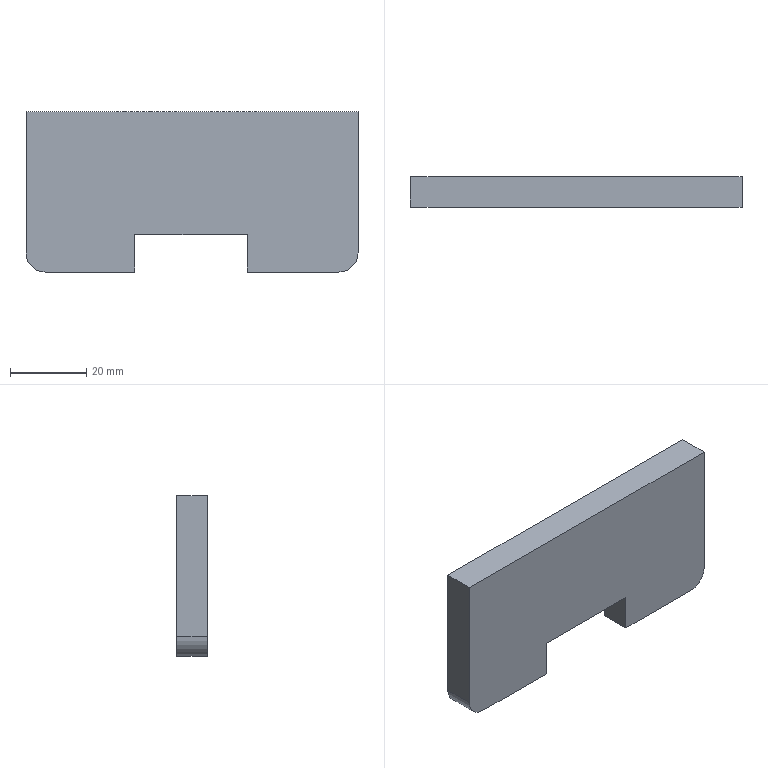Part | STEP file | 1 solid | 12 faces | box 87 x 8 x 41.949 mm | volume 26801 mm3 | plane 10 | cylinder 2 | commonest cylinder face diameters 10 x2
STEP:
#1=CARTESIAN_POINT('',(0.,0.,0.));
#2=DIRECTION('',(0.,0.,1.));
#3=DIRECTION('',(1.,0.,0.));
#4=AXIS2_PLACEMENT_3D('',#1,#2,#3);
#5=CARTESIAN_POINT('',(-4.362,37.,-78.42));
#6=VERTEX_POINT('',#5);
#7=CARTESIAN_POINT('',(-28.362,37.,-78.42));
#8=VERTEX_POINT('',#7);
#9=CARTESIAN_POINT('',(-42.862,37.,-78.42));
#10=DIRECTION('',(-1.,0.,0.));
#11=VECTOR('',#10,1.);
#12=LINE('',#9,#11);
#13=CARTESIAN_POINT('',(-42.862,37.,-64.47));
#14=DIRECTION('',(0.,1.,0.));
#15=DIRECTION('',(0.,0.,1.));
#16=AXIS2_PLACEMENT_3D('',#13,#14,#15);
#17=PLANE('',#16);
#18=CARTESIAN_POINT('',(-13.949,0.));
#19=DIRECTION('',(0.,-1.));
#20=VECTOR('',#19,1.);
#21=LINE('',#18,#20);
#22=(GEOMETRIC_REPRESENTATION_CONTEXT(2)PARAMETRIC_REPRESENTATION_CONTEXT()REPRESENTATION_CONTEXT('',''));
#23=DEFINITIONAL_REPRESENTATION('',(#21),#22);
#24=PCURVE('',#17,#23);
#25=CARTESIAN_POINT('',(-7.863,-150.,-78.42));
#26=DIRECTION('',(0.,0.,-1.));
#27=DIRECTION('',(-1.,0.,0.));
#28=AXIS2_PLACEMENT_3D('',#25,#26,#27);
#29=PLANE('',#28);
#30=CARTESIAN_POINT('',(35.,187.));
#31=DIRECTION('',(1.,0.));
#32=VECTOR('',#31,1.);
#33=LINE('',#30,#32);
#34=(GEOMETRIC_REPRESENTATION_CONTEXT(2)PARAMETRIC_REPRESENTATION_CONTEXT()REPRESENTATION_CONTEXT('',''));
#35=DEFINITIONAL_REPRESENTATION('',(#33),#34);
#36=PCURVE('',#29,#35);
#37=SURFACE_CURVE('',#12,(#24,#36),.PCURVE_S1.);
#38=EDGE_CURVE('',#6,#8,#37,.T.);
#39=ORIENTED_EDGE('',*,*,#38,.F.);
#40=CARTESIAN_POINT('',(0.6375,37.,-73.42));
#41=VERTEX_POINT('',#40);
#42=CARTESIAN_POINT('',(-4.362,37.,-73.42));
#43=DIRECTION('',(0.,-1.,0.));
#44=DIRECTION('',(0.,0.,1.));
#45=AXIS2_PLACEMENT_3D('',#42,#43,#44);
#46=CIRCLE('',#45,5.);
#47=CARTESIAN_POINT('',(-3.949,38.5));
#48=CARTESIAN_POINT('',(-3.949,29.84));
#49=CARTESIAN_POINT('',(-11.449,34.17));
#50=CARTESIAN_POINT('',(-18.949,38.5));
#51=CARTESIAN_POINT('',(-11.449,42.83));
#52=CARTESIAN_POINT('',(-3.949,47.16));
#53=CARTESIAN_POINT('',(-3.949,38.5));
#54=(BOUNDED_CURVE()B_SPLINE_CURVE(2,(#47,#48,#49,#50,#51,#52,#53),.UNSPECIFIED.,.T.,.F.)B_SPLINE_CURVE_WITH_KNOTS((1,2,2,2,2,1),(-2.094,0.,2.094,4.189,6.283,8.378),.UNSPECIFIED.)CURVE()GEOMETRIC_REPRESENTATION_ITEM()RATIONAL_B_SPLINE_CURVE((1.,0.5,1.,0.5,1.,0.5,1.))REPRESENTATION_ITEM(''));
#55=(GEOMETRIC_REPRESENTATION_CONTEXT(2)PARAMETRIC_REPRESENTATION_CONTEXT()REPRESENTATION_CONTEXT('',''));
#56=DEFINITIONAL_REPRESENTATION('',(#54),#55);
#57=PCURVE('',#17,#56);
#58=CARTESIAN_POINT('',(-4.362,37.,-73.42));
#59=DIRECTION('',(0.,-1.,0.));
#60=DIRECTION('',(0.,0.,-1.));
#61=AXIS2_PLACEMENT_3D('',#58,#59,#60);
#62=CYLINDRICAL_SURFACE('',#61,5.);
#63=CARTESIAN_POINT('',(-3.142,0.));
#64=DIRECTION('',(1.,0.));
#65=VECTOR('',#64,1.);
#66=LINE('',#63,#65);
#67=(GEOMETRIC_REPRESENTATION_CONTEXT(2)PARAMETRIC_REPRESENTATION_CONTEXT()REPRESENTATION_CONTEXT('',''));
#68=DEFINITIONAL_REPRESENTATION('',(#66),#67);
#69=PCURVE('',#62,#68);
#70=SURFACE_CURVE('',#46,(#57,#69),.PCURVE_S1.);
#71=EDGE_CURVE('',#6,#41,#70,.T.);
#72=ORIENTED_EDGE('',*,*,#71,.T.);
#73=CARTESIAN_POINT('',(0.6375,37.,-36.47));
#74=VERTEX_POINT('',#73);
#75=CARTESIAN_POINT('',(0.6375,37.,-64.47));
#76=DIRECTION('',(0.,0.,1.));
#77=VECTOR('',#76,1.);
#78=LINE('',#75,#77);
#79=CARTESIAN_POINT('',(0.,43.5));
#80=DIRECTION('',(1.,0.));
#81=VECTOR('',#80,1.);
#82=LINE('',#79,#81);
#83=(GEOMETRIC_REPRESENTATION_CONTEXT(2)PARAMETRIC_REPRESENTATION_CONTEXT()REPRESENTATION_CONTEXT('',''));
#84=DEFINITIONAL_REPRESENTATION('',(#82),#83);
#85=PCURVE('',#17,#84);
#86=CARTESIAN_POINT('',(0.6375,37.,-92.47));
#87=DIRECTION('',(-1.,0.,0.));
#88=DIRECTION('',(0.,0.,1.));
#89=AXIS2_PLACEMENT_3D('',#86,#87,#88);
#90=PLANE('',#89);
#91=CARTESIAN_POINT('',(28.,0.));
#92=DIRECTION('',(1.,0.));
#93=VECTOR('',#92,1.);
#94=LINE('',#91,#93);
#95=(GEOMETRIC_REPRESENTATION_CONTEXT(2)PARAMETRIC_REPRESENTATION_CONTEXT()REPRESENTATION_CONTEXT('',''));
#96=DEFINITIONAL_REPRESENTATION('',(#94),#95);
#97=PCURVE('',#90,#96);
#98=SURFACE_CURVE('',#78,(#85,#97),.PCURVE_S1.);
#99=EDGE_CURVE('',#41,#74,#98,.T.);
#100=ORIENTED_EDGE('',*,*,#99,.T.);
#101=CARTESIAN_POINT('',(-86.362,37.,-36.47));
#102=VERTEX_POINT('',#101);
#103=CARTESIAN_POINT('',(-42.862,37.,-36.47));
#104=DIRECTION('',(-1.,0.,0.));
#105=VECTOR('',#104,1.);
#106=LINE('',#103,#105);
#107=CARTESIAN_POINT('',(28.,0.));
#108=DIRECTION('',(0.,-1.));
#109=VECTOR('',#108,1.);
#110=LINE('',#107,#109);
#111=(GEOMETRIC_REPRESENTATION_CONTEXT(2)PARAMETRIC_REPRESENTATION_CONTEXT()REPRESENTATION_CONTEXT('',''));
#112=DEFINITIONAL_REPRESENTATION('',(#110),#111);
#113=PCURVE('',#17,#112);
#114=CARTESIAN_POINT('',(-42.862,0.,-36.47));
#115=DIRECTION('',(0.,0.,1.));
#116=DIRECTION('',(1.,0.,0.));
#117=AXIS2_PLACEMENT_3D('',#114,#115,#116);
#118=PLANE('',#117);
#119=CARTESIAN_POINT('',(0.,37.));
#120=DIRECTION('',(-1.,0.));
#121=VECTOR('',#120,1.);
#122=LINE('',#119,#121);
#123=(GEOMETRIC_REPRESENTATION_CONTEXT(2)PARAMETRIC_REPRESENTATION_CONTEXT()REPRESENTATION_CONTEXT('',''));
#124=DEFINITIONAL_REPRESENTATION('',(#122),#123);
#125=PCURVE('',#118,#124);
#126=SURFACE_CURVE('',#106,(#113,#125),.PCURVE_S1.);
#127=EDGE_CURVE('',#74,#102,#126,.T.);
#128=ORIENTED_EDGE('',*,*,#127,.T.);
#129=CARTESIAN_POINT('',(-86.362,37.,-73.42));
#130=VERTEX_POINT('',#129);
#131=CARTESIAN_POINT('',(-86.362,37.,-64.47));
#132=DIRECTION('',(0.,0.,-1.));
#133=VECTOR('',#132,1.);
#134=LINE('',#131,#133);
#135=CARTESIAN_POINT('',(0.,-43.5));
#136=DIRECTION('',(-1.,0.));
#137=VECTOR('',#136,1.);
#138=LINE('',#135,#137);
#139=(GEOMETRIC_REPRESENTATION_CONTEXT(2)PARAMETRIC_REPRESENTATION_CONTEXT()REPRESENTATION_CONTEXT('',''));
#140=DEFINITIONAL_REPRESENTATION('',(#138),#139);
#141=PCURVE('',#17,#140);
#142=CARTESIAN_POINT('',(-86.362,37.,-92.47));
#143=DIRECTION('',(1.,0.,0.));
#144=DIRECTION('',(0.,0.,-1.));
#145=AXIS2_PLACEMENT_3D('',#142,#143,#144);
#146=PLANE('',#145);
#147=CARTESIAN_POINT('',(-28.,0.));
#148=DIRECTION('',(1.,0.));
#149=VECTOR('',#148,1.);
#150=LINE('',#147,#149);
#151=(GEOMETRIC_REPRESENTATION_CONTEXT(2)PARAMETRIC_REPRESENTATION_CONTEXT()REPRESENTATION_CONTEXT('',''));
#152=DEFINITIONAL_REPRESENTATION('',(#150),#151);
#153=PCURVE('',#146,#152);
#154=SURFACE_CURVE('',#134,(#141,#153),.PCURVE_S1.);
#155=EDGE_CURVE('',#102,#130,#154,.T.);
#156=ORIENTED_EDGE('',*,*,#155,.T.);
#157=CARTESIAN_POINT('',(-81.362,37.,-78.42));
#158=VERTEX_POINT('',#157);
#159=CARTESIAN_POINT('',(-81.362,37.,-73.42));
#160=DIRECTION('',(0.,-1.,0.));
#161=DIRECTION('',(0.,0.,1.));
#162=AXIS2_PLACEMENT_3D('',#159,#160,#161);
#163=CIRCLE('',#162,5.);
#164=CARTESIAN_POINT('',(-3.949,-38.5));
#165=CARTESIAN_POINT('',(-3.949,-47.16));
#166=CARTESIAN_POINT('',(-11.449,-42.83));
#167=CARTESIAN_POINT('',(-18.949,-38.5));
#168=CARTESIAN_POINT('',(-11.449,-34.17));
#169=CARTESIAN_POINT('',(-3.949,-29.84));
#170=CARTESIAN_POINT('',(-3.949,-38.5));
#171=(BOUNDED_CURVE()B_SPLINE_CURVE(2,(#164,#165,#166,#167,#168,#169,#170),.UNSPECIFIED.,.T.,.F.)B_SPLINE_CURVE_WITH_KNOTS((1,2,2,2,2,1),(-2.094,0.,2.094,4.189,6.283,8.378),.UNSPECIFIED.)CURVE()GEOMETRIC_REPRESENTATION_ITEM()RATIONAL_B_SPLINE_CURVE((1.,0.5,1.,0.5,1.,0.5,1.))REPRESENTATION_ITEM(''));
#172=(GEOMETRIC_REPRESENTATION_CONTEXT(2)PARAMETRIC_REPRESENTATION_CONTEXT()REPRESENTATION_CONTEXT('',''));
#173=DEFINITIONAL_REPRESENTATION('',(#171),#172);
#174=PCURVE('',#17,#173);
#175=CARTESIAN_POINT('',(-81.362,37.,-73.42));
#176=DIRECTION('',(0.,1.,0.));
#177=DIRECTION('',(0.,0.,1.));
#178=AXIS2_PLACEMENT_3D('',#175,#176,#177);
#179=CYLINDRICAL_SURFACE('',#178,5.);
#180=CARTESIAN_POINT('',(6.283,0.));
#181=DIRECTION('',(-1.,0.));
#182=VECTOR('',#181,1.);
#183=LINE('',#180,#182);
#184=(GEOMETRIC_REPRESENTATION_CONTEXT(2)PARAMETRIC_REPRESENTATION_CONTEXT()REPRESENTATION_CONTEXT('',''));
#185=DEFINITIONAL_REPRESENTATION('',(#183),#184);
#186=PCURVE('',#179,#185);
#187=SURFACE_CURVE('',#163,(#174,#186),.PCURVE_S1.);
#188=EDGE_CURVE('',#130,#158,#187,.T.);
#189=ORIENTED_EDGE('',*,*,#188,.T.);
#190=CARTESIAN_POINT('',(-57.862,37.,-78.42));
#191=VERTEX_POINT('',#190);
#192=CARTESIAN_POINT('',(-42.862,37.,-78.42));
#193=DIRECTION('',(-1.,0.,0.));
#194=VECTOR('',#193,1.);
#195=LINE('',#192,#194);
#196=CARTESIAN_POINT('',(-13.949,0.));
#197=DIRECTION('',(0.,-1.));
#198=VECTOR('',#197,1.);
#199=LINE('',#196,#198);
#200=(GEOMETRIC_REPRESENTATION_CONTEXT(2)PARAMETRIC_REPRESENTATION_CONTEXT()REPRESENTATION_CONTEXT('',''));
#201=DEFINITIONAL_REPRESENTATION('',(#199),#200);
#202=PCURVE('',#17,#201);
#203=CARTESIAN_POINT('',(-7.863,-150.,-78.42));
#204=DIRECTION('',(0.,0.,-1.));
#205=DIRECTION('',(-1.,0.,0.));
#206=AXIS2_PLACEMENT_3D('',#203,#204,#205);
#207=PLANE('',#206);
#208=CARTESIAN_POINT('',(35.,187.));
#209=DIRECTION('',(1.,0.));
#210=VECTOR('',#209,1.);
#211=LINE('',#208,#210);
#212=(GEOMETRIC_REPRESENTATION_CONTEXT(2)PARAMETRIC_REPRESENTATION_CONTEXT()REPRESENTATION_CONTEXT('',''));
#213=DEFINITIONAL_REPRESENTATION('',(#211),#212);
#214=PCURVE('',#207,#213);
#215=SURFACE_CURVE('',#195,(#202,#214),.PCURVE_S1.);
#216=EDGE_CURVE('',#191,#158,#215,.T.);
#217=ORIENTED_EDGE('',*,*,#216,.F.);
#218=CARTESIAN_POINT('',(-57.862,37.,-68.634));
#219=VERTEX_POINT('',#218);
#220=CARTESIAN_POINT('',(-57.862,37.,-64.47));
#221=DIRECTION('',(0.,0.,1.));
#222=VECTOR('',#221,1.);
#223=LINE('',#220,#222);
#224=CARTESIAN_POINT('',(0.,-15.));
#225=DIRECTION('',(1.,0.));
#226=VECTOR('',#225,1.);
#227=LINE('',#224,#226);
#228=(GEOMETRIC_REPRESENTATION_CONTEXT(2)PARAMETRIC_REPRESENTATION_CONTEXT()REPRESENTATION_CONTEXT('',''));
#229=DEFINITIONAL_REPRESENTATION('',(#227),#228);
#230=PCURVE('',#17,#229);
#231=CARTESIAN_POINT('',(-57.862,-50.076,-69.634));
#232=DIRECTION('',(-1.,0.,0.));
#233=DIRECTION('',(0.,0.,1.));
#234=AXIS2_PLACEMENT_3D('',#231,#232,#233);
#235=PLANE('',#234);
#236=CARTESIAN_POINT('',(5.163,87.076));
#237=DIRECTION('',(1.,0.));
#238=VECTOR('',#237,1.);
#239=LINE('',#236,#238);
#240=(GEOMETRIC_REPRESENTATION_CONTEXT(2)PARAMETRIC_REPRESENTATION_CONTEXT()REPRESENTATION_CONTEXT('',''));
#241=DEFINITIONAL_REPRESENTATION('',(#239),#240);
#242=PCURVE('',#235,#241);
#243=SURFACE_CURVE('',#223,(#230,#242),.PCURVE_S1.);
#244=EDGE_CURVE('',#191,#219,#243,.T.);
#245=ORIENTED_EDGE('',*,*,#244,.T.);
#246=CARTESIAN_POINT('',(-28.362,37.,-68.634));
#247=VERTEX_POINT('',#246);
#248=CARTESIAN_POINT('',(-42.862,37.,-68.634));
#249=DIRECTION('',(-1.,0.,0.));
#250=VECTOR('',#249,1.);
#251=LINE('',#248,#250);
#252=CARTESIAN_POINT('',(-4.163,0.));
#253=DIRECTION('',(0.,-1.));
#254=VECTOR('',#253,1.);
#255=LINE('',#252,#254);
#256=(GEOMETRIC_REPRESENTATION_CONTEXT(2)PARAMETRIC_REPRESENTATION_CONTEXT()REPRESENTATION_CONTEXT('',''));
#257=DEFINITIONAL_REPRESENTATION('',(#255),#256);
#258=PCURVE('',#17,#257);
#259=CARTESIAN_POINT('',(-43.112,-50.076,-68.634));
#260=DIRECTION('',(0.,0.,-1.));
#261=DIRECTION('',(-1.,0.,0.));
#262=AXIS2_PLACEMENT_3D('',#259,#260,#261);
#263=PLANE('',#262);
#264=CARTESIAN_POINT('',(-0.25,87.076));
#265=DIRECTION('',(1.,0.));
#266=VECTOR('',#265,1.);
#267=LINE('',#264,#266);
#268=(GEOMETRIC_REPRESENTATION_CONTEXT(2)PARAMETRIC_REPRESENTATION_CONTEXT()REPRESENTATION_CONTEXT('',''));
#269=DEFINITIONAL_REPRESENTATION('',(#267),#268);
#270=PCURVE('',#263,#269);
#271=SURFACE_CURVE('',#251,(#258,#270),.PCURVE_S1.);
#272=EDGE_CURVE('',#247,#219,#271,.T.);
#273=ORIENTED_EDGE('',*,*,#272,.F.);
#274=CARTESIAN_POINT('',(-28.362,37.,-69.634));
#275=DIRECTION('',(0.,0.,-1.));
#276=VECTOR('',#275,1.);
#277=LINE('',#274,#276);
#278=CARTESIAN_POINT('',(-5.163,14.5));
#279=DIRECTION('',(-1.,0.));
#280=VECTOR('',#279,1.);
#281=LINE('',#278,#280);
#282=(GEOMETRIC_REPRESENTATION_CONTEXT(2)PARAMETRIC_REPRESENTATION_CONTEXT()REPRESENTATION_CONTEXT('',''));
#283=DEFINITIONAL_REPRESENTATION('',(#281),#282);
#284=PCURVE('',#17,#283);
#285=CARTESIAN_POINT('',(-28.362,-50.076,-69.634));
#286=DIRECTION('',(1.,0.,0.));
#287=DIRECTION('',(0.,0.,-1.));
#288=AXIS2_PLACEMENT_3D('',#285,#286,#287);
#289=PLANE('',#288);
#290=CARTESIAN_POINT('',(0.,87.076));
#291=DIRECTION('',(1.,0.));
#292=VECTOR('',#291,1.);
#293=LINE('',#290,#292);
#294=(GEOMETRIC_REPRESENTATION_CONTEXT(2)PARAMETRIC_REPRESENTATION_CONTEXT()REPRESENTATION_CONTEXT('',''));
#295=DEFINITIONAL_REPRESENTATION('',(#293),#294);
#296=PCURVE('',#289,#295);
#297=SURFACE_CURVE('',#277,(#284,#296),.PCURVE_S1.);
#298=EDGE_CURVE('',#247,#8,#297,.T.);
#299=ORIENTED_EDGE('',*,*,#298,.T.);
#300=EDGE_LOOP('',(#39,#72,#100,#128,#156,#189,#217,#245,#273,#299));
#301=FACE_BOUND('',#300,.T.);
#302=ADVANCED_FACE('',(#301),#17,.F.);
#303=ORIENTED_EDGE('',*,*,#216,.T.);
#304=CARTESIAN_POINT('',(-81.362,45.,-78.42));
#305=VERTEX_POINT('',#304);
#306=CARTESIAN_POINT('',(-81.362,45.,-78.42));
#307=DIRECTION('',(0.,1.,0.));
#308=VECTOR('',#307,1.);
#309=LINE('',#306,#308);
#310=CARTESIAN_POINT('',(73.5,195.));
#311=DIRECTION('',(0.,1.));
#312=VECTOR('',#311,1.);
#313=LINE('',#310,#312);
#314=(GEOMETRIC_REPRESENTATION_CONTEXT(2)PARAMETRIC_REPRESENTATION_CONTEXT()REPRESENTATION_CONTEXT('',''));
#315=DEFINITIONAL_REPRESENTATION('',(#313),#314);
#316=PCURVE('',#207,#315);
#317=CARTESIAN_POINT('',(3.142,8.));
#318=DIRECTION('',(0.,1.));
#319=VECTOR('',#318,1.);
#320=LINE('',#317,#319);
#321=(GEOMETRIC_REPRESENTATION_CONTEXT(2)PARAMETRIC_REPRESENTATION_CONTEXT()REPRESENTATION_CONTEXT('',''));
#322=DEFINITIONAL_REPRESENTATION('',(#320),#321);
#323=PCURVE('',#179,#322);
#324=SURFACE_CURVE('',#309,(#316,#323),.PCURVE_S1.);
#325=EDGE_CURVE('',#158,#305,#324,.T.);
#326=ORIENTED_EDGE('',*,*,#325,.T.);
#327=CARTESIAN_POINT('',(-57.862,45.,-78.42));
#328=VERTEX_POINT('',#327);
#329=CARTESIAN_POINT('',(-42.862,45.,-78.42));
#330=DIRECTION('',(-1.,0.,0.));
#331=VECTOR('',#330,1.);
#332=LINE('',#329,#331);
#333=CARTESIAN_POINT('',(35.,195.));
#334=DIRECTION('',(1.,0.));
#335=VECTOR('',#334,1.);
#336=LINE('',#333,#335);
#337=(GEOMETRIC_REPRESENTATION_CONTEXT(2)PARAMETRIC_REPRESENTATION_CONTEXT()REPRESENTATION_CONTEXT('',''));
#338=DEFINITIONAL_REPRESENTATION('',(#336),#337);
#339=PCURVE('',#207,#338);
#340=CARTESIAN_POINT('',(-42.862,45.,-64.47));
#341=DIRECTION('',(0.,1.,0.));
#342=DIRECTION('',(0.,0.,1.));
#343=AXIS2_PLACEMENT_3D('',#340,#341,#342);
#344=PLANE('',#343);
#345=CARTESIAN_POINT('',(-13.949,0.));
#346=DIRECTION('',(0.,-1.));
#347=VECTOR('',#346,1.);
#348=LINE('',#345,#347);
#349=(GEOMETRIC_REPRESENTATION_CONTEXT(2)PARAMETRIC_REPRESENTATION_CONTEXT()REPRESENTATION_CONTEXT('',''));
#350=DEFINITIONAL_REPRESENTATION('',(#348),#349);
#351=PCURVE('',#344,#350);
#352=SURFACE_CURVE('',#332,(#339,#351),.PCURVE_S1.);
#353=EDGE_CURVE('',#328,#305,#352,.T.);
#354=ORIENTED_EDGE('',*,*,#353,.F.);
#355=CARTESIAN_POINT('',(-57.862,-50.076,-78.42));
#356=DIRECTION('',(0.,-1.,0.));
#357=VECTOR('',#356,1.);
#358=LINE('',#355,#357);
#359=CARTESIAN_POINT('',(50.,99.924));
#360=DIRECTION('',(0.,-1.));
#361=VECTOR('',#360,1.);
#362=LINE('',#359,#361);
#363=(GEOMETRIC_REPRESENTATION_CONTEXT(2)PARAMETRIC_REPRESENTATION_CONTEXT()REPRESENTATION_CONTEXT('',''));
#364=DEFINITIONAL_REPRESENTATION('',(#362),#363);
#365=PCURVE('',#207,#364);
#366=CARTESIAN_POINT('',(-8.786,0.));
#367=DIRECTION('',(0.,-1.));
#368=VECTOR('',#367,1.);
#369=LINE('',#366,#368);
#370=(GEOMETRIC_REPRESENTATION_CONTEXT(2)PARAMETRIC_REPRESENTATION_CONTEXT()REPRESENTATION_CONTEXT('',''));
#371=DEFINITIONAL_REPRESENTATION('',(#369),#370);
#372=PCURVE('',#235,#371);
#373=SURFACE_CURVE('',#358,(#365,#372),.PCURVE_S1.);
#374=EDGE_CURVE('',#328,#191,#373,.T.);
#375=ORIENTED_EDGE('',*,*,#374,.T.);
#376=EDGE_LOOP('',(#303,#326,#354,#375));
#377=FACE_BOUND('',#376,.T.);
#378=ADVANCED_FACE('',(#377),#207,.T.);
#379=CARTESIAN_POINT('',(-4.362,45.,-78.42));
#380=VERTEX_POINT('',#379);
#381=CARTESIAN_POINT('',(-28.362,45.,-78.42));
#382=VERTEX_POINT('',#381);
#383=CARTESIAN_POINT('',(-42.862,45.,-78.42));
#384=DIRECTION('',(-1.,0.,0.));
#385=VECTOR('',#384,1.);
#386=LINE('',#383,#385);
#387=CARTESIAN_POINT('',(35.,195.));
#388=DIRECTION('',(1.,0.));
#389=VECTOR('',#388,1.);
#390=LINE('',#387,#389);
#391=(GEOMETRIC_REPRESENTATION_CONTEXT(2)PARAMETRIC_REPRESENTATION_CONTEXT()REPRESENTATION_CONTEXT('',''));
#392=DEFINITIONAL_REPRESENTATION('',(#390),#391);
#393=PCURVE('',#29,#392);
#394=CARTESIAN_POINT('',(-13.949,0.));
#395=DIRECTION('',(0.,-1.));
#396=VECTOR('',#395,1.);
#397=LINE('',#394,#396);
#398=(GEOMETRIC_REPRESENTATION_CONTEXT(2)PARAMETRIC_REPRESENTATION_CONTEXT()REPRESENTATION_CONTEXT('',''));
#399=DEFINITIONAL_REPRESENTATION('',(#397),#398);
#400=PCURVE('',#344,#399);
#401=SURFACE_CURVE('',#386,(#393,#400),.PCURVE_S1.);
#402=EDGE_CURVE('',#380,#382,#401,.T.);
#403=ORIENTED_EDGE('',*,*,#402,.F.);
#404=CARTESIAN_POINT('',(-4.362,37.,-78.42));
#405=DIRECTION('',(0.,-1.,0.));
#406=VECTOR('',#405,1.);
#407=LINE('',#404,#406);
#408=CARTESIAN_POINT('',(-3.5,187.));
#409=DIRECTION('',(0.,-1.));
#410=VECTOR('',#409,1.);
#411=LINE('',#408,#410);
#412=(GEOMETRIC_REPRESENTATION_CONTEXT(2)PARAMETRIC_REPRESENTATION_CONTEXT()REPRESENTATION_CONTEXT('',''));
#413=DEFINITIONAL_REPRESENTATION('',(#411),#412);
#414=PCURVE('',#29,#413);
#415=CARTESIAN_POINT('',(0.,0.));
#416=DIRECTION('',(0.,1.));
#417=VECTOR('',#416,1.);
#418=LINE('',#415,#417);
#419=(GEOMETRIC_REPRESENTATION_CONTEXT(2)PARAMETRIC_REPRESENTATION_CONTEXT()REPRESENTATION_CONTEXT('',''));
#420=DEFINITIONAL_REPRESENTATION('',(#418),#419);
#421=PCURVE('',#62,#420);
#422=SURFACE_CURVE('',#407,(#414,#421),.PCURVE_S1.);
#423=EDGE_CURVE('',#380,#6,#422,.T.);
#424=ORIENTED_EDGE('',*,*,#423,.T.);
#425=ORIENTED_EDGE('',*,*,#38,.T.);
#426=CARTESIAN_POINT('',(-28.362,-150.,-78.42));
#427=DIRECTION('',(0.,1.,0.));
#428=VECTOR('',#427,1.);
#429=LINE('',#426,#428);
#430=CARTESIAN_POINT('',(20.5,0.));
#431=DIRECTION('',(0.,1.));
#432=VECTOR('',#431,1.);
#433=LINE('',#430,#432);
#434=(GEOMETRIC_REPRESENTATION_CONTEXT(2)PARAMETRIC_REPRESENTATION_CONTEXT()REPRESENTATION_CONTEXT('',''));
#435=DEFINITIONAL_REPRESENTATION('',(#433),#434);
#436=PCURVE('',#29,#435);
#437=CARTESIAN_POINT('',(8.786,-99.924));
#438=DIRECTION('',(0.,1.));
#439=VECTOR('',#438,1.);
#440=LINE('',#437,#439);
#441=(GEOMETRIC_REPRESENTATION_CONTEXT(2)PARAMETRIC_REPRESENTATION_CONTEXT()REPRESENTATION_CONTEXT('',''));
#442=DEFINITIONAL_REPRESENTATION('',(#440),#441);
#443=PCURVE('',#289,#442);
#444=SURFACE_CURVE('',#429,(#436,#443),.PCURVE_S1.);
#445=EDGE_CURVE('',#8,#382,#444,.T.);
#446=ORIENTED_EDGE('',*,*,#445,.T.);
#447=EDGE_LOOP('',(#403,#424,#425,#446));
#448=FACE_BOUND('',#447,.T.);
#449=ADVANCED_FACE('',(#448),#29,.T.);
#450=CARTESIAN_POINT('',(0.6375,45.,-73.42));
#451=VERTEX_POINT('',#450);
#452=CARTESIAN_POINT('',(0.6375,45.,-36.47));
#453=VERTEX_POINT('',#452);
#454=CARTESIAN_POINT('',(0.6375,45.,-64.47));
#455=DIRECTION('',(0.,0.,1.));
#456=VECTOR('',#455,1.);
#457=LINE('',#454,#456);
#458=CARTESIAN_POINT('',(0.,43.5));
#459=DIRECTION('',(1.,0.));
#460=VECTOR('',#459,1.);
#461=LINE('',#458,#460);
#462=(GEOMETRIC_REPRESENTATION_CONTEXT(2)PARAMETRIC_REPRESENTATION_CONTEXT()REPRESENTATION_CONTEXT('',''));
#463=DEFINITIONAL_REPRESENTATION('',(#461),#462);
#464=PCURVE('',#344,#463);
#465=CARTESIAN_POINT('',(28.,8.));
#466=DIRECTION('',(1.,0.));
#467=VECTOR('',#466,1.);
#468=LINE('',#465,#467);
#469=(GEOMETRIC_REPRESENTATION_CONTEXT(2)PARAMETRIC_REPRESENTATION_CONTEXT()REPRESENTATION_CONTEXT('',''));
#470=DEFINITIONAL_REPRESENTATION('',(#468),#469);
#471=PCURVE('',#90,#470);
#472=SURFACE_CURVE('',#457,(#464,#471),.PCURVE_S1.);
#473=EDGE_CURVE('',#451,#453,#472,.T.);
#474=ORIENTED_EDGE('',*,*,#473,.F.);
#475=CARTESIAN_POINT('',(-4.362,45.,-73.42));
#476=DIRECTION('',(0.,1.,0.));
#477=DIRECTION('',(0.,0.,1.));
#478=AXIS2_PLACEMENT_3D('',#475,#476,#477);
#479=CIRCLE('',#478,5.);
#480=CARTESIAN_POINT('',(-8.949,38.5));
#481=DIRECTION('',(1.,0.));
#482=AXIS2_PLACEMENT_2D('',#480,#481);
#483=CIRCLE('',#482,5.);
#484=(GEOMETRIC_REPRESENTATION_CONTEXT(2)PARAMETRIC_REPRESENTATION_CONTEXT()REPRESENTATION_CONTEXT('',''));
#485=DEFINITIONAL_REPRESENTATION('',(#483),#484);
#486=PCURVE('',#344,#485);
#487=CARTESIAN_POINT('',(3.142,-8.));
#488=DIRECTION('',(-1.,0.));
#489=VECTOR('',#488,1.);
#490=LINE('',#487,#489);
#491=(GEOMETRIC_REPRESENTATION_CONTEXT(2)PARAMETRIC_REPRESENTATION_CONTEXT()REPRESENTATION_CONTEXT('',''));
#492=DEFINITIONAL_REPRESENTATION('',(#490),#491);
#493=PCURVE('',#62,#492);
#494=SURFACE_CURVE('',#479,(#486,#493),.PCURVE_S1.);
#495=EDGE_CURVE('',#451,#380,#494,.T.);
#496=ORIENTED_EDGE('',*,*,#495,.T.);
#497=ORIENTED_EDGE('',*,*,#402,.T.);
#498=CARTESIAN_POINT('',(-28.362,45.,-68.634));
#499=VERTEX_POINT('',#498);
#500=CARTESIAN_POINT('',(-28.362,45.,-69.634));
#501=DIRECTION('',(0.,0.,-1.));
#502=VECTOR('',#501,1.);
#503=LINE('',#500,#502);
#504=CARTESIAN_POINT('',(-5.163,14.5));
#505=DIRECTION('',(-1.,0.));
#506=VECTOR('',#505,1.);
#507=LINE('',#504,#506);
#508=(GEOMETRIC_REPRESENTATION_CONTEXT(2)PARAMETRIC_REPRESENTATION_CONTEXT()REPRESENTATION_CONTEXT('',''));
#509=DEFINITIONAL_REPRESENTATION('',(#507),#508);
#510=PCURVE('',#344,#509);
#511=CARTESIAN_POINT('',(0.,95.076));
#512=DIRECTION('',(1.,0.));
#513=VECTOR('',#512,1.);
#514=LINE('',#511,#513);
#515=(GEOMETRIC_REPRESENTATION_CONTEXT(2)PARAMETRIC_REPRESENTATION_CONTEXT()REPRESENTATION_CONTEXT('',''));
#516=DEFINITIONAL_REPRESENTATION('',(#514),#515);
#517=PCURVE('',#289,#516);
#518=SURFACE_CURVE('',#503,(#510,#517),.PCURVE_S1.);
#519=EDGE_CURVE('',#499,#382,#518,.T.);
#520=ORIENTED_EDGE('',*,*,#519,.F.);
#521=CARTESIAN_POINT('',(-57.862,45.,-68.634));
#522=VERTEX_POINT('',#521);
#523=CARTESIAN_POINT('',(-42.862,45.,-68.634));
#524=DIRECTION('',(-1.,0.,0.));
#525=VECTOR('',#524,1.);
#526=LINE('',#523,#525);
#527=CARTESIAN_POINT('',(-4.163,0.));
#528=DIRECTION('',(0.,-1.));
#529=VECTOR('',#528,1.);
#530=LINE('',#527,#529);
#531=(GEOMETRIC_REPRESENTATION_CONTEXT(2)PARAMETRIC_REPRESENTATION_CONTEXT()REPRESENTATION_CONTEXT('',''));
#532=DEFINITIONAL_REPRESENTATION('',(#530),#531);
#533=PCURVE('',#344,#532);
#534=CARTESIAN_POINT('',(-0.25,95.076));
#535=DIRECTION('',(1.,0.));
#536=VECTOR('',#535,1.);
#537=LINE('',#534,#536);
#538=(GEOMETRIC_REPRESENTATION_CONTEXT(2)PARAMETRIC_REPRESENTATION_CONTEXT()REPRESENTATION_CONTEXT('',''));
#539=DEFINITIONAL_REPRESENTATION('',(#537),#538);
#540=PCURVE('',#263,#539);
#541=SURFACE_CURVE('',#526,(#533,#540),.PCURVE_S1.);
#542=EDGE_CURVE('',#499,#522,#541,.T.);
#543=ORIENTED_EDGE('',*,*,#542,.T.);
#544=CARTESIAN_POINT('',(-57.862,45.,-64.47));
#545=DIRECTION('',(0.,0.,1.));
#546=VECTOR('',#545,1.);
#547=LINE('',#544,#546);
#548=CARTESIAN_POINT('',(0.,-15.));
#549=DIRECTION('',(1.,0.));
#550=VECTOR('',#549,1.);
#551=LINE('',#548,#550);
#552=(GEOMETRIC_REPRESENTATION_CONTEXT(2)PARAMETRIC_REPRESENTATION_CONTEXT()REPRESENTATION_CONTEXT('',''));
#553=DEFINITIONAL_REPRESENTATION('',(#551),#552);
#554=PCURVE('',#344,#553);
#555=CARTESIAN_POINT('',(5.163,95.076));
#556=DIRECTION('',(1.,0.));
#557=VECTOR('',#556,1.);
#558=LINE('',#555,#557);
#559=(GEOMETRIC_REPRESENTATION_CONTEXT(2)PARAMETRIC_REPRESENTATION_CONTEXT()REPRESENTATION_CONTEXT('',''));
#560=DEFINITIONAL_REPRESENTATION('',(#558),#559);
#561=PCURVE('',#235,#560);
#562=SURFACE_CURVE('',#547,(#554,#561),.PCURVE_S1.);
#563=EDGE_CURVE('',#328,#522,#562,.T.);
#564=ORIENTED_EDGE('',*,*,#563,.F.);
#565=ORIENTED_EDGE('',*,*,#353,.T.);
#566=CARTESIAN_POINT('',(-86.362,45.,-73.42));
#567=VERTEX_POINT('',#566);
#568=CARTESIAN_POINT('',(-81.362,45.,-73.42));
#569=DIRECTION('',(0.,1.,0.));
#570=DIRECTION('',(0.,0.,1.));
#571=AXIS2_PLACEMENT_3D('',#568,#569,#570);
#572=CIRCLE('',#571,5.);
#573=CARTESIAN_POINT('',(-8.949,-38.5));
#574=DIRECTION('',(1.,0.));
#575=AXIS2_PLACEMENT_2D('',#573,#574);
#576=CIRCLE('',#575,5.);
#577=(GEOMETRIC_REPRESENTATION_CONTEXT(2)PARAMETRIC_REPRESENTATION_CONTEXT()REPRESENTATION_CONTEXT('',''));
#578=DEFINITIONAL_REPRESENTATION('',(#576),#577);
#579=PCURVE('',#344,#578);
#580=CARTESIAN_POINT('',(0.,8.));
#581=DIRECTION('',(1.,0.));
#582=VECTOR('',#581,1.);
#583=LINE('',#580,#582);
#584=(GEOMETRIC_REPRESENTATION_CONTEXT(2)PARAMETRIC_REPRESENTATION_CONTEXT()REPRESENTATION_CONTEXT('',''));
#585=DEFINITIONAL_REPRESENTATION('',(#583),#584);
#586=PCURVE('',#179,#585);
#587=SURFACE_CURVE('',#572,(#579,#586),.PCURVE_S1.);
#588=EDGE_CURVE('',#305,#567,#587,.T.);
#589=ORIENTED_EDGE('',*,*,#588,.T.);
#590=CARTESIAN_POINT('',(-86.362,45.,-36.47));
#591=VERTEX_POINT('',#590);
#592=CARTESIAN_POINT('',(-86.362,45.,-64.47));
#593=DIRECTION('',(0.,0.,-1.));
#594=VECTOR('',#593,1.);
#595=LINE('',#592,#594);
#596=CARTESIAN_POINT('',(0.,-43.5));
#597=DIRECTION('',(-1.,0.));
#598=VECTOR('',#597,1.);
#599=LINE('',#596,#598);
#600=(GEOMETRIC_REPRESENTATION_CONTEXT(2)PARAMETRIC_REPRESENTATION_CONTEXT()REPRESENTATION_CONTEXT('',''));
#601=DEFINITIONAL_REPRESENTATION('',(#599),#600);
#602=PCURVE('',#344,#601);
#603=CARTESIAN_POINT('',(-28.,8.));
#604=DIRECTION('',(1.,0.));
#605=VECTOR('',#604,1.);
#606=LINE('',#603,#605);
#607=(GEOMETRIC_REPRESENTATION_CONTEXT(2)PARAMETRIC_REPRESENTATION_CONTEXT()REPRESENTATION_CONTEXT('',''));
#608=DEFINITIONAL_REPRESENTATION('',(#606),#607);
#609=PCURVE('',#146,#608);
#610=SURFACE_CURVE('',#595,(#602,#609),.PCURVE_S1.);
#611=EDGE_CURVE('',#591,#567,#610,.T.);
#612=ORIENTED_EDGE('',*,*,#611,.F.);
#613=CARTESIAN_POINT('',(-42.862,45.,-36.47));
#614=DIRECTION('',(-1.,0.,0.));
#615=VECTOR('',#614,1.);
#616=LINE('',#613,#615);
#617=CARTESIAN_POINT('',(28.,0.));
#618=DIRECTION('',(0.,-1.));
#619=VECTOR('',#618,1.);
#620=LINE('',#617,#619);
#621=(GEOMETRIC_REPRESENTATION_CONTEXT(2)PARAMETRIC_REPRESENTATION_CONTEXT()REPRESENTATION_CONTEXT('',''));
#622=DEFINITIONAL_REPRESENTATION('',(#620),#621);
#623=PCURVE('',#344,#622);
#624=CARTESIAN_POINT('',(0.,45.));
#625=DIRECTION('',(-1.,0.));
#626=VECTOR('',#625,1.);
#627=LINE('',#624,#626);
#628=(GEOMETRIC_REPRESENTATION_CONTEXT(2)PARAMETRIC_REPRESENTATION_CONTEXT()REPRESENTATION_CONTEXT('',''));
#629=DEFINITIONAL_REPRESENTATION('',(#627),#628);
#630=PCURVE('',#118,#629);
#631=SURFACE_CURVE('',#616,(#623,#630),.PCURVE_S1.);
#632=EDGE_CURVE('',#453,#591,#631,.T.);
#633=ORIENTED_EDGE('',*,*,#632,.F.);
#634=EDGE_LOOP('',(#474,#496,#497,#520,#543,#564,#565,#589,#612,#633));
#635=FACE_BOUND('',#634,.T.);
#636=ADVANCED_FACE('',(#635),#344,.T.);
#637=ORIENTED_EDGE('',*,*,#632,.T.);
#638=CARTESIAN_POINT('',(-86.362,37.,-36.47));
#639=DIRECTION('',(0.,1.,0.));
#640=VECTOR('',#639,1.);
#641=LINE('',#638,#640);
#642=CARTESIAN_POINT('',(-43.5,37.));
#643=DIRECTION('',(0.,1.));
#644=VECTOR('',#643,1.);
#645=LINE('',#642,#644);
#646=(GEOMETRIC_REPRESENTATION_CONTEXT(2)PARAMETRIC_REPRESENTATION_CONTEXT()REPRESENTATION_CONTEXT('',''));
#647=DEFINITIONAL_REPRESENTATION('',(#645),#646);
#648=PCURVE('',#118,#647);
#649=CARTESIAN_POINT('',(-56.,0.));
#650=DIRECTION('',(0.,1.));
#651=VECTOR('',#650,1.);
#652=LINE('',#649,#651);
#653=(GEOMETRIC_REPRESENTATION_CONTEXT(2)PARAMETRIC_REPRESENTATION_CONTEXT()REPRESENTATION_CONTEXT('',''));
#654=DEFINITIONAL_REPRESENTATION('',(#652),#653);
#655=PCURVE('',#146,#654);
#656=SURFACE_CURVE('',#641,(#648,#655),.PCURVE_S1.);
#657=EDGE_CURVE('',#102,#591,#656,.T.);
#658=ORIENTED_EDGE('',*,*,#657,.F.);
#659=ORIENTED_EDGE('',*,*,#127,.F.);
#660=CARTESIAN_POINT('',(0.6375,0.,-36.47));
#661=DIRECTION('',(0.,1.,0.));
#662=VECTOR('',#661,1.);
#663=LINE('',#660,#662);
#664=CARTESIAN_POINT('',(43.5,0.));
#665=DIRECTION('',(0.,1.));
#666=VECTOR('',#665,1.);
#667=LINE('',#664,#666);
#668=(GEOMETRIC_REPRESENTATION_CONTEXT(2)PARAMETRIC_REPRESENTATION_CONTEXT()REPRESENTATION_CONTEXT('',''));
#669=DEFINITIONAL_REPRESENTATION('',(#667),#668);
#670=PCURVE('',#118,#669);
#671=CARTESIAN_POINT('',(56.,-37.));
#672=DIRECTION('',(0.,1.));
#673=VECTOR('',#672,1.);
#674=LINE('',#671,#673);
#675=(GEOMETRIC_REPRESENTATION_CONTEXT(2)PARAMETRIC_REPRESENTATION_CONTEXT()REPRESENTATION_CONTEXT('',''));
#676=DEFINITIONAL_REPRESENTATION('',(#674),#675);
#677=PCURVE('',#90,#676);
#678=SURFACE_CURVE('',#663,(#670,#677),.PCURVE_S1.);
#679=EDGE_CURVE('',#74,#453,#678,.T.);
#680=ORIENTED_EDGE('',*,*,#679,.T.);
#681=EDGE_LOOP('',(#637,#658,#659,#680));
#682=FACE_BOUND('',#681,.T.);
#683=ADVANCED_FACE('',(#682),#118,.T.);
#684=ORIENTED_EDGE('',*,*,#611,.T.);
#685=CARTESIAN_POINT('',(-86.362,37.,-73.42));
#686=DIRECTION('',(0.,-1.,0.));
#687=VECTOR('',#686,1.);
#688=LINE('',#685,#687);
#689=CARTESIAN_POINT('',(-19.051,0.));
#690=DIRECTION('',(0.,-1.));
#691=VECTOR('',#690,1.);
#692=LINE('',#689,#691);
#693=(GEOMETRIC_REPRESENTATION_CONTEXT(2)PARAMETRIC_REPRESENTATION_CONTEXT()REPRESENTATION_CONTEXT('',''));
#694=DEFINITIONAL_REPRESENTATION('',(#692),#693);
#695=PCURVE('',#146,#694);
#696=CARTESIAN_POINT('',(4.712,0.));
#697=DIRECTION('',(0.,-1.));
#698=VECTOR('',#697,1.);
#699=LINE('',#696,#698);
#700=(GEOMETRIC_REPRESENTATION_CONTEXT(2)PARAMETRIC_REPRESENTATION_CONTEXT()REPRESENTATION_CONTEXT('',''));
#701=DEFINITIONAL_REPRESENTATION('',(#699),#700);
#702=PCURVE('',#179,#701);
#703=SURFACE_CURVE('',#688,(#695,#702),.PCURVE_S1.);
#704=EDGE_CURVE('',#567,#130,#703,.T.);
#705=ORIENTED_EDGE('',*,*,#704,.T.);
#706=ORIENTED_EDGE('',*,*,#155,.F.);
#707=ORIENTED_EDGE('',*,*,#657,.T.);
#708=EDGE_LOOP('',(#684,#705,#706,#707));
#709=FACE_BOUND('',#708,.T.);
#710=ADVANCED_FACE('',(#709),#146,.F.);
#711=ORIENTED_EDGE('',*,*,#99,.F.);
#712=CARTESIAN_POINT('',(0.6375,45.,-73.42));
#713=DIRECTION('',(0.,1.,0.));
#714=VECTOR('',#713,1.);
#715=LINE('',#712,#714);
#716=CARTESIAN_POINT('',(19.051,8.));
#717=DIRECTION('',(0.,1.));
#718=VECTOR('',#717,1.);
#719=LINE('',#716,#718);
#720=(GEOMETRIC_REPRESENTATION_CONTEXT(2)PARAMETRIC_REPRESENTATION_CONTEXT()REPRESENTATION_CONTEXT('',''));
#721=DEFINITIONAL_REPRESENTATION('',(#719),#720);
#722=PCURVE('',#90,#721);
#723=CARTESIAN_POINT('',(1.571,-8.));
#724=DIRECTION('',(0.,-1.));
#725=VECTOR('',#724,1.);
#726=LINE('',#723,#725);
#727=(GEOMETRIC_REPRESENTATION_CONTEXT(2)PARAMETRIC_REPRESENTATION_CONTEXT()REPRESENTATION_CONTEXT('',''));
#728=DEFINITIONAL_REPRESENTATION('',(#726),#727);
#729=PCURVE('',#62,#728);
#730=SURFACE_CURVE('',#715,(#722,#729),.PCURVE_S1.);
#731=EDGE_CURVE('',#41,#451,#730,.T.);
#732=ORIENTED_EDGE('',*,*,#731,.T.);
#733=ORIENTED_EDGE('',*,*,#473,.T.);
#734=ORIENTED_EDGE('',*,*,#679,.F.);
#735=EDGE_LOOP('',(#711,#732,#733,#734));
#736=FACE_BOUND('',#735,.T.);
#737=ADVANCED_FACE('',(#736),#90,.F.);
#738=ORIENTED_EDGE('',*,*,#244,.F.);
#739=ORIENTED_EDGE('',*,*,#374,.F.);
#740=ORIENTED_EDGE('',*,*,#563,.T.);
#741=CARTESIAN_POINT('',(-57.862,-50.076,-68.634));
#742=DIRECTION('',(0.,1.,0.));
#743=VECTOR('',#742,1.);
#744=LINE('',#741,#743);
#745=CARTESIAN_POINT('',(1.,0.));
#746=DIRECTION('',(0.,1.));
#747=VECTOR('',#746,1.);
#748=LINE('',#745,#747);
#749=(GEOMETRIC_REPRESENTATION_CONTEXT(2)PARAMETRIC_REPRESENTATION_CONTEXT()REPRESENTATION_CONTEXT('',''));
#750=DEFINITIONAL_REPRESENTATION('',(#748),#749);
#751=PCURVE('',#235,#750);
#752=CARTESIAN_POINT('',(14.75,0.));
#753=DIRECTION('',(0.,1.));
#754=VECTOR('',#753,1.);
#755=LINE('',#752,#754);
#756=(GEOMETRIC_REPRESENTATION_CONTEXT(2)PARAMETRIC_REPRESENTATION_CONTEXT()REPRESENTATION_CONTEXT('',''));
#757=DEFINITIONAL_REPRESENTATION('',(#755),#756);
#758=PCURVE('',#263,#757);
#759=SURFACE_CURVE('',#744,(#751,#758),.PCURVE_S1.);
#760=EDGE_CURVE('',#219,#522,#759,.T.);
#761=ORIENTED_EDGE('',*,*,#760,.F.);
#762=EDGE_LOOP('',(#738,#739,#740,#761));
#763=FACE_BOUND('',#762,.T.);
#764=ADVANCED_FACE('',(#763),#235,.F.);
#765=ORIENTED_EDGE('',*,*,#445,.F.);
#766=ORIENTED_EDGE('',*,*,#298,.F.);
#767=CARTESIAN_POINT('',(-28.362,-50.076,-68.634));
#768=DIRECTION('',(0.,1.,0.));
#769=VECTOR('',#768,1.);
#770=LINE('',#767,#769);
#771=CARTESIAN_POINT('',(-1.,0.));
#772=DIRECTION('',(0.,1.));
#773=VECTOR('',#772,1.);
#774=LINE('',#771,#773);
#775=(GEOMETRIC_REPRESENTATION_CONTEXT(2)PARAMETRIC_REPRESENTATION_CONTEXT()REPRESENTATION_CONTEXT('',''));
#776=DEFINITIONAL_REPRESENTATION('',(#774),#775);
#777=PCURVE('',#289,#776);
#778=CARTESIAN_POINT('',(-14.75,0.));
#779=DIRECTION('',(0.,1.));
#780=VECTOR('',#779,1.);
#781=LINE('',#778,#780);
#782=(GEOMETRIC_REPRESENTATION_CONTEXT(2)PARAMETRIC_REPRESENTATION_CONTEXT()REPRESENTATION_CONTEXT('',''));
#783=DEFINITIONAL_REPRESENTATION('',(#781),#782);
#784=PCURVE('',#263,#783);
#785=SURFACE_CURVE('',#770,(#777,#784),.PCURVE_S1.);
#786=EDGE_CURVE('',#247,#499,#785,.T.);
#787=ORIENTED_EDGE('',*,*,#786,.T.);
#788=ORIENTED_EDGE('',*,*,#519,.T.);
#789=EDGE_LOOP('',(#765,#766,#787,#788));
#790=FACE_BOUND('',#789,.T.);
#791=ADVANCED_FACE('',(#790),#289,.F.);
#792=ORIENTED_EDGE('',*,*,#272,.T.);
#793=ORIENTED_EDGE('',*,*,#760,.T.);
#794=ORIENTED_EDGE('',*,*,#542,.F.);
#795=ORIENTED_EDGE('',*,*,#786,.F.);
#796=EDGE_LOOP('',(#792,#793,#794,#795));
#797=FACE_BOUND('',#796,.T.);
#798=ADVANCED_FACE('',(#797),#263,.T.);
#799=ORIENTED_EDGE('',*,*,#71,.F.);
#800=ORIENTED_EDGE('',*,*,#423,.F.);
#801=ORIENTED_EDGE('',*,*,#495,.F.);
#802=ORIENTED_EDGE('',*,*,#731,.F.);
#803=EDGE_LOOP('',(#799,#800,#801,#802));
#804=FACE_BOUND('',#803,.T.);
#805=ADVANCED_FACE('',(#804),#62,.T.);
#806=ORIENTED_EDGE('',*,*,#588,.F.);
#807=ORIENTED_EDGE('',*,*,#325,.F.);
#808=ORIENTED_EDGE('',*,*,#188,.F.);
#809=ORIENTED_EDGE('',*,*,#704,.F.);
#810=EDGE_LOOP('',(#806,#807,#808,#809));
#811=FACE_BOUND('',#810,.T.);
#812=ADVANCED_FACE('',(#811),#179,.T.);
#813=CLOSED_SHELL('',(#302,#378,#449,#636,#683,#710,#737,#764,#791,#798,#805,#812));
#814=MANIFOLD_SOLID_BREP('',#813);
#815=(LENGTH_UNIT()NAMED_UNIT(*)SI_UNIT(.MILLI.,.METRE.));
#816=UNCERTAINTY_MEASURE_WITH_UNIT(LENGTH_MEASURE(0.0000001),#815,'','');
#817=(NAMED_UNIT(*)PLANE_ANGLE_UNIT()SI_UNIT($,.RADIAN.));
#818=(NAMED_UNIT(*)SI_UNIT($,.STERADIAN.)SOLID_ANGLE_UNIT());
#819=(GEOMETRIC_REPRESENTATION_CONTEXT(3)GLOBAL_UNCERTAINTY_ASSIGNED_CONTEXT((#816))GLOBAL_UNIT_ASSIGNED_CONTEXT((#815,#817,#818))REPRESENTATION_CONTEXT('',''));
#820=ADVANCED_BREP_SHAPE_REPRESENTATION('',(#4,#814),#819);